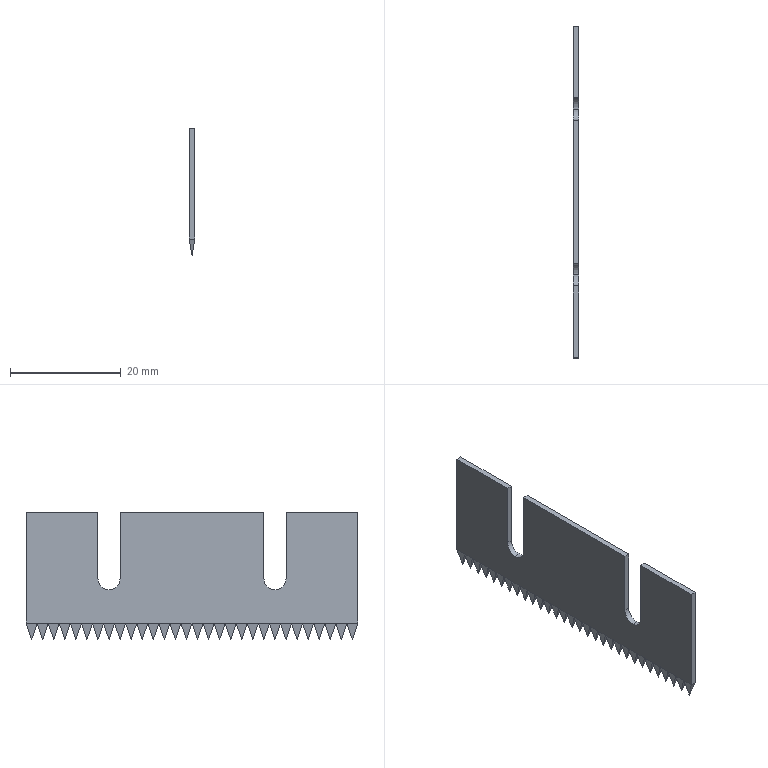Part | STEP file | 1 solid | 135 faces | box 1 x 60 x 23 mm | volume 1151 mm3 | plane 131 | cylinder 4 | commonest cylinder face diameters 4 x4